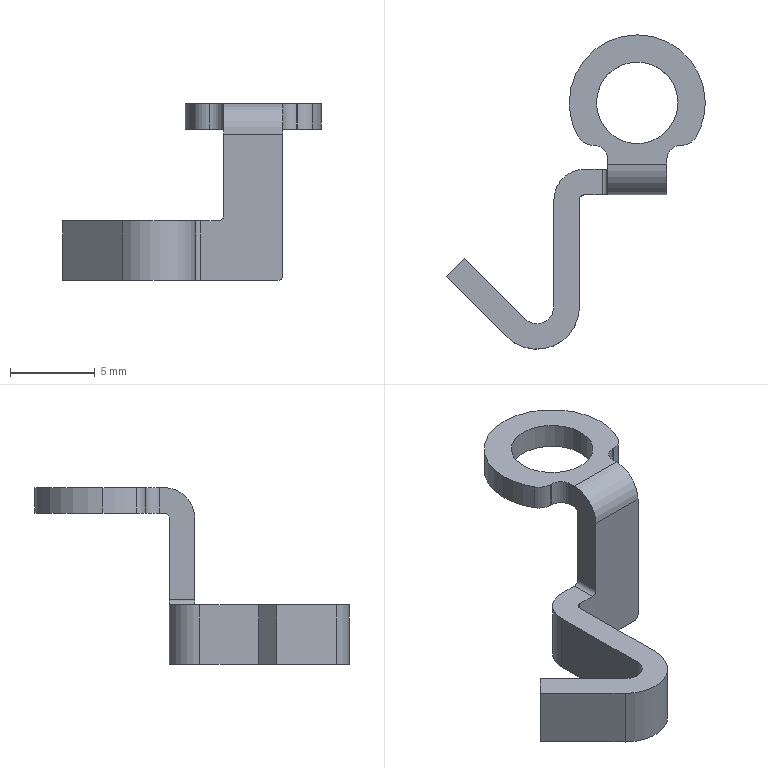Part | STEP file | TQ-DD-1105-THTerminalB1010_デフォルト | 1 solid | 32 faces | box 15.207 x 18.483 x 10.4 mm | volume 194.982 mm3 | cylinder 17 | plane 15 | commonest cylinder face diameters 0.6 x4 2 x3 8 x3 1.6 x2 3.6 x2 4.8 x2
STEP:
#1=CARTESIAN_POINT('',(2.4,0.,0.));
#2=VERTEX_POINT('',#1);
#3=CARTESIAN_POINT('',(-2.4,0.,0.));
#4=VERTEX_POINT('',#3);
#5=CARTESIAN_POINT('',(0.,0.,0.));
#6=DIRECTION('',(0.,0.,-1.));
#7=DIRECTION('',(1.,0.,0.));
#8=AXIS2_PLACEMENT_3D('',#5,#6,#7);
#9=CIRCLE('',#8,2.4);
#10=EDGE_CURVE('',#2,#4,#9,.T.);
#11=ORIENTED_EDGE('',*,*,#10,.T.);
#12=CARTESIAN_POINT('',(-2.4,0.,1.5));
#13=VERTEX_POINT('',#12);
#14=CARTESIAN_POINT('',(-2.4,0.,0.75));
#15=DIRECTION('',(0.,0.,1.));
#16=VECTOR('',#15,1000.);
#17=LINE('',#14,#16);
#18=EDGE_CURVE('',#4,#13,#17,.T.);
#19=ORIENTED_EDGE('',*,*,#18,.T.);
#20=CARTESIAN_POINT('',(2.4,0.,1.5));
#21=VERTEX_POINT('',#20);
#22=CARTESIAN_POINT('',(0.,0.,1.5));
#23=DIRECTION('',(0.,0.,-1.));
#24=DIRECTION('',(1.,0.,0.));
#25=AXIS2_PLACEMENT_3D('',#22,#23,#24);
#26=CIRCLE('',#25,2.4);
#27=EDGE_CURVE('',#21,#13,#26,.T.);
#28=ORIENTED_EDGE('',*,*,#27,.F.);
#29=CARTESIAN_POINT('',(2.4,0.,0.75));
#30=DIRECTION('',(0.,0.,1.));
#31=VECTOR('',#30,1000.);
#32=LINE('',#29,#31);
#33=EDGE_CURVE('',#2,#21,#32,.T.);
#34=ORIENTED_EDGE('',*,*,#33,.F.);
#35=EDGE_LOOP('',(#11,#19,#28,#34));
#36=FACE_OUTER_BOUND('',#35,.T.);
#37=CARTESIAN_POINT('',(0.,0.,0.75));
#38=DIRECTION('',(0.,0.,1.));
#39=DIRECTION('',(1.,0.,0.));
#40=AXIS2_PLACEMENT_3D('',#37,#38,#39);
#41=CYLINDRICAL_SURFACE('',#40,2.4);
#42=ADVANCED_FACE('',(#36),#41,.F.);
#43=CARTESIAN_POINT('',(4.,0.,0.));
#44=VERTEX_POINT('',#43);
#45=CARTESIAN_POINT('',(-4.,0.,0.));
#46=VERTEX_POINT('',#45);
#47=CARTESIAN_POINT('',(0.,0.,0.));
#48=DIRECTION('',(0.,0.,1.));
#49=DIRECTION('',(1.,0.,0.));
#50=AXIS2_PLACEMENT_3D('',#47,#48,#49);
#51=CIRCLE('',#50,4.);
#52=EDGE_CURVE('',#44,#46,#51,.T.);
#53=ORIENTED_EDGE('',*,*,#52,.T.);
#54=CARTESIAN_POINT('',(-4.,0.,1.5));
#55=VERTEX_POINT('',#54);
#56=CARTESIAN_POINT('',(-4.,0.,0.75));
#57=DIRECTION('',(0.,0.,1.));
#58=VECTOR('',#57,1000.);
#59=LINE('',#56,#58);
#60=EDGE_CURVE('',#46,#55,#59,.T.);
#61=ORIENTED_EDGE('',*,*,#60,.T.);
#62=CARTESIAN_POINT('',(4.,0.,1.5));
#63=VERTEX_POINT('',#62);
#64=CARTESIAN_POINT('',(0.,0.,1.5));
#65=DIRECTION('',(0.,0.,1.));
#66=DIRECTION('',(1.,0.,0.));
#67=AXIS2_PLACEMENT_3D('',#64,#65,#66);
#68=CIRCLE('',#67,4.);
#69=EDGE_CURVE('',#63,#55,#68,.T.);
#70=ORIENTED_EDGE('',*,*,#69,.F.);
#71=CARTESIAN_POINT('',(4.,0.,0.75));
#72=DIRECTION('',(0.,0.,1.));
#73=VECTOR('',#72,1000.);
#74=LINE('',#71,#73);
#75=EDGE_CURVE('',#44,#63,#74,.T.);
#76=ORIENTED_EDGE('',*,*,#75,.F.);
#77=EDGE_LOOP('',(#53,#61,#70,#76));
#78=FACE_OUTER_BOUND('',#77,.T.);
#79=CARTESIAN_POINT('',(0.,0.,0.75));
#80=DIRECTION('',(0.,0.,1.));
#81=DIRECTION('',(1.,0.,0.));
#82=AXIS2_PLACEMENT_3D('',#79,#80,#81);
#83=CYLINDRICAL_SURFACE('',#82,4.);
#84=ADVANCED_FACE('',(#78),#83,.T.);
#85=CARTESIAN_POINT('',(3.464,-2.,0.));
#86=VERTEX_POINT('',#85);
#87=CARTESIAN_POINT('',(0.,0.,0.));
#88=DIRECTION('',(0.,0.,1.));
#89=DIRECTION('',(1.,0.,0.));
#90=AXIS2_PLACEMENT_3D('',#87,#88,#89);
#91=CIRCLE('',#90,4.);
#92=EDGE_CURVE('',#86,#44,#91,.T.);
#93=ORIENTED_EDGE('',*,*,#92,.T.);
#94=ORIENTED_EDGE('',*,*,#75,.T.);
#95=CARTESIAN_POINT('',(3.464,-2.,1.5));
#96=VERTEX_POINT('',#95);
#97=CARTESIAN_POINT('',(0.,0.,1.5));
#98=DIRECTION('',(0.,0.,1.));
#99=DIRECTION('',(1.,0.,0.));
#100=AXIS2_PLACEMENT_3D('',#97,#98,#99);
#101=CIRCLE('',#100,4.);
#102=EDGE_CURVE('',#96,#63,#101,.T.);
#103=ORIENTED_EDGE('',*,*,#102,.F.);
#104=CARTESIAN_POINT('',(3.464,-2.,0.75));
#105=DIRECTION('',(0.,0.,1.));
#106=VECTOR('',#105,1000.);
#107=LINE('',#104,#106);
#108=EDGE_CURVE('',#86,#96,#107,.T.);
#109=ORIENTED_EDGE('',*,*,#108,.F.);
#110=EDGE_LOOP('',(#93,#94,#103,#109));
#111=FACE_OUTER_BOUND('',#110,.T.);
#112=CARTESIAN_POINT('',(0.,0.,0.75));
#113=DIRECTION('',(0.,0.,1.));
#114=DIRECTION('',(1.,0.,0.));
#115=AXIS2_PLACEMENT_3D('',#112,#113,#114);
#116=CYLINDRICAL_SURFACE('',#115,4.);
#117=ADVANCED_FACE('',(#111),#116,.T.);
#118=CARTESIAN_POINT('',(-3.104,-3.9,-8.9));
#119=VERTEX_POINT('',#118);
#120=CARTESIAN_POINT('',(1.45,-3.9,-8.9));
#121=VERTEX_POINT('',#120);
#122=CARTESIAN_POINT('',(0.,-3.9,-8.9));
#123=DIRECTION('',(1.,0.,0.));
#124=VECTOR('',#123,1000.);
#125=LINE('',#122,#124);
#126=EDGE_CURVE('',#119,#121,#125,.T.);
#127=ORIENTED_EDGE('',*,*,#126,.F.);
#128=CARTESIAN_POINT('',(-3.104,-3.9,-5.4));
#129=VERTEX_POINT('',#128);
#130=CARTESIAN_POINT('',(-3.104,-3.9,1.5));
#131=DIRECTION('',(0.,0.,-1.));
#132=VECTOR('',#131,1000.);
#133=LINE('',#130,#132);
#134=EDGE_CURVE('',#129,#119,#133,.T.);
#135=ORIENTED_EDGE('',*,*,#134,.F.);
#136=CARTESIAN_POINT('',(-2.05,-3.9,-5.4));
#137=VERTEX_POINT('',#136);
#138=CARTESIAN_POINT('',(0.,-3.9,-5.4));
#139=DIRECTION('',(1.,0.,0.));
#140=VECTOR('',#139,1000.);
#141=LINE('',#138,#140);
#142=EDGE_CURVE('',#129,#137,#141,.T.);
#143=ORIENTED_EDGE('',*,*,#142,.T.);
#144=CARTESIAN_POINT('',(-1.75,-3.9,-5.1));
#145=VERTEX_POINT('',#144);
#146=CARTESIAN_POINT('',(-2.05,-3.9,-5.1));
#147=DIRECTION('',(0.,-1.,0.));
#148=DIRECTION('',(0.,0.,1.));
#149=AXIS2_PLACEMENT_3D('',#146,#147,#148);
#150=CIRCLE('',#149,0.3);
#151=EDGE_CURVE('',#137,#145,#150,.T.);
#152=ORIENTED_EDGE('',*,*,#151,.T.);
#153=CARTESIAN_POINT('',(-1.75,-3.9,-0.3));
#154=VERTEX_POINT('',#153);
#155=CARTESIAN_POINT('',(-1.75,-3.9,1.5));
#156=DIRECTION('',(0.,0.,-1.));
#157=VECTOR('',#156,1000.);
#158=LINE('',#155,#157);
#159=EDGE_CURVE('',#154,#145,#158,.T.);
#160=ORIENTED_EDGE('',*,*,#159,.F.);
#161=CARTESIAN_POINT('',(1.75,-3.9,-0.3));
#162=VERTEX_POINT('',#161);
#163=CARTESIAN_POINT('',(0.,-3.9,-0.3));
#164=DIRECTION('',(-1.,0.,0.));
#165=VECTOR('',#164,1000.);
#166=LINE('',#163,#165);
#167=EDGE_CURVE('',#162,#154,#166,.T.);
#168=ORIENTED_EDGE('',*,*,#167,.F.);
#169=CARTESIAN_POINT('',(1.75,-3.9,-8.6));
#170=VERTEX_POINT('',#169);
#171=CARTESIAN_POINT('',(1.75,-3.9,1.5));
#172=DIRECTION('',(0.,0.,1.));
#173=VECTOR('',#172,1000.);
#174=LINE('',#171,#173);
#175=EDGE_CURVE('',#170,#162,#174,.T.);
#176=ORIENTED_EDGE('',*,*,#175,.F.);
#177=CARTESIAN_POINT('',(1.45,-3.9,-8.6));
#178=DIRECTION('',(0.,-1.,0.));
#179=DIRECTION('',(0.,0.,1.));
#180=AXIS2_PLACEMENT_3D('',#177,#178,#179);
#181=CIRCLE('',#180,0.3);
#182=EDGE_CURVE('',#121,#170,#181,.T.);
#183=ORIENTED_EDGE('',*,*,#182,.F.);
#184=EDGE_LOOP('',(#127,#135,#143,#152,#160,#168,#176,#183));
#185=FACE_OUTER_BOUND('',#184,.T.);
#186=CARTESIAN_POINT('',(0.,-3.9,1.5));
#187=DIRECTION('',(0.,-1.,0.));
#188=DIRECTION('',(0.,0.,-1.));
#189=AXIS2_PLACEMENT_3D('',#186,#187,#188);
#190=PLANE('',#189);
#191=ADVANCED_FACE('',(#185),#190,.F.);
#192=ORIENTED_EDGE('',*,*,#126,.T.);
#193=CARTESIAN_POINT('',(1.45,-5.4,-8.9));
#194=VERTEX_POINT('',#193);
#195=CARTESIAN_POINT('',(1.45,-5.4,-8.9));
#196=DIRECTION('',(0.,-1.,0.));
#197=VECTOR('',#196,1000.);
#198=LINE('',#195,#197);
#199=EDGE_CURVE('',#121,#194,#198,.T.);
#200=ORIENTED_EDGE('',*,*,#199,.T.);
#201=CARTESIAN_POINT('',(-3.104,-5.4,-8.9));
#202=VERTEX_POINT('',#201);
#203=CARTESIAN_POINT('',(0.,-5.4,-8.9));
#204=DIRECTION('',(-1.,0.,0.));
#205=VECTOR('',#204,1000.);
#206=LINE('',#203,#205);
#207=EDGE_CURVE('',#194,#202,#206,.T.);
#208=ORIENTED_EDGE('',*,*,#207,.T.);
#209=CARTESIAN_POINT('',(-3.404,-5.7,-8.9));
#210=VERTEX_POINT('',#209);
#211=CARTESIAN_POINT('',(-3.104,-5.7,-8.9));
#212=DIRECTION('',(0.,0.,1.));
#213=DIRECTION('',(-1.,0.,0.));
#214=AXIS2_PLACEMENT_3D('',#211,#212,#213);
#215=CIRCLE('',#214,0.3);
#216=EDGE_CURVE('',#202,#210,#215,.T.);
#217=ORIENTED_EDGE('',*,*,#216,.T.);
#218=CARTESIAN_POINT('',(-3.404,-11.983,-8.9));
#219=VERTEX_POINT('',#218);
#220=CARTESIAN_POINT('',(-3.404,-5.4,-8.9));
#221=DIRECTION('',(0.,-1.,0.));
#222=VECTOR('',#221,1000.);
#223=LINE('',#220,#222);
#224=EDGE_CURVE('',#210,#219,#223,.T.);
#225=ORIENTED_EDGE('',*,*,#224,.T.);
#226=CARTESIAN_POINT('',(-7.672,-13.751,-8.9));
#227=VERTEX_POINT('',#226);
#228=CARTESIAN_POINT('',(-5.904,-11.983,-8.9));
#229=DIRECTION('',(0.,0.,-1.));
#230=DIRECTION('',(-1.,0.,0.));
#231=AXIS2_PLACEMENT_3D('',#228,#229,#230);
#232=CIRCLE('',#231,2.5);
#233=EDGE_CURVE('',#219,#227,#232,.T.);
#234=ORIENTED_EDGE('',*,*,#233,.T.);
#235=CARTESIAN_POINT('',(-11.207,-10.216,-8.9));
#236=VERTEX_POINT('',#235);
#237=CARTESIAN_POINT('',(-7.672,-13.751,-8.9));
#238=DIRECTION('',(-0.7071,0.7071,0.));
#239=VECTOR('',#238,1000.);
#240=LINE('',#237,#239);
#241=EDGE_CURVE('',#227,#236,#240,.T.);
#242=ORIENTED_EDGE('',*,*,#241,.T.);
#243=CARTESIAN_POINT('',(-10.147,-9.155,-8.9));
#244=VERTEX_POINT('',#243);
#245=CARTESIAN_POINT('',(-10.147,-9.155,-8.9));
#246=DIRECTION('',(-0.7071,-0.7071,0.));
#247=VECTOR('',#246,1000.);
#248=LINE('',#245,#247);
#249=EDGE_CURVE('',#244,#236,#248,.T.);
#250=ORIENTED_EDGE('',*,*,#249,.F.);
#251=CARTESIAN_POINT('',(-6.611,-12.691,-8.9));
#252=VERTEX_POINT('',#251);
#253=CARTESIAN_POINT('',(-10.147,-9.155,-8.9));
#254=DIRECTION('',(0.7071,-0.7071,0.));
#255=VECTOR('',#254,1000.);
#256=LINE('',#253,#255);
#257=EDGE_CURVE('',#244,#252,#256,.T.);
#258=ORIENTED_EDGE('',*,*,#257,.T.);
#259=CARTESIAN_POINT('',(-4.904,-11.983,-8.9));
#260=VERTEX_POINT('',#259);
#261=CARTESIAN_POINT('',(-5.904,-11.983,-8.9));
#262=DIRECTION('',(0.,0.,1.));
#263=DIRECTION('',(-1.,0.,0.));
#264=AXIS2_PLACEMENT_3D('',#261,#262,#263);
#265=CIRCLE('',#264,1.);
#266=EDGE_CURVE('',#252,#260,#265,.T.);
#267=ORIENTED_EDGE('',*,*,#266,.T.);
#268=CARTESIAN_POINT('',(-4.904,-5.7,-8.9));
#269=VERTEX_POINT('',#268);
#270=CARTESIAN_POINT('',(-4.904,-5.4,-8.9));
#271=DIRECTION('',(0.,1.,0.));
#272=VECTOR('',#271,1000.);
#273=LINE('',#270,#272);
#274=EDGE_CURVE('',#260,#269,#273,.T.);
#275=ORIENTED_EDGE('',*,*,#274,.T.);
#276=CARTESIAN_POINT('',(-3.104,-5.7,-8.9));
#277=DIRECTION('',(0.,0.,-1.));
#278=DIRECTION('',(-1.,0.,0.));
#279=AXIS2_PLACEMENT_3D('',#276,#277,#278);
#280=CIRCLE('',#279,1.8);
#281=EDGE_CURVE('',#269,#119,#280,.T.);
#282=ORIENTED_EDGE('',*,*,#281,.T.);
#283=EDGE_LOOP('',(#192,#200,#208,#217,#225,#234,#242,#250,#258,#267,#275,#282));
#284=FACE_OUTER_BOUND('',#283,.T.);
#285=CARTESIAN_POINT('',(0.,-5.4,-8.9));
#286=DIRECTION('',(0.,0.,-1.));
#287=DIRECTION('',(-1.,0.,0.));
#288=AXIS2_PLACEMENT_3D('',#285,#286,#287);
#289=PLANE('',#288);
#290=ADVANCED_FACE('',(#284),#289,.T.);
#291=ORIENTED_EDGE('',*,*,#281,.F.);
#292=CARTESIAN_POINT('',(-4.904,-5.7,-5.4));
#293=VERTEX_POINT('',#292);
#294=CARTESIAN_POINT('',(-4.904,-5.7,-7.15));
#295=DIRECTION('',(0.,0.,1.));
#296=VECTOR('',#295,1000.);
#297=LINE('',#294,#296);
#298=EDGE_CURVE('',#269,#293,#297,.T.);
#299=ORIENTED_EDGE('',*,*,#298,.T.);
#300=CARTESIAN_POINT('',(-3.104,-5.7,-5.4));
#301=DIRECTION('',(0.,0.,-1.));
#302=DIRECTION('',(-1.,0.,0.));
#303=AXIS2_PLACEMENT_3D('',#300,#301,#302);
#304=CIRCLE('',#303,1.8);
#305=EDGE_CURVE('',#293,#129,#304,.T.);
#306=ORIENTED_EDGE('',*,*,#305,.T.);
#307=ORIENTED_EDGE('',*,*,#134,.T.);
#308=EDGE_LOOP('',(#291,#299,#306,#307));
#309=FACE_OUTER_BOUND('',#308,.T.);
#310=CARTESIAN_POINT('',(-3.104,-5.7,-7.15));
#311=DIRECTION('',(0.,0.,-1.));
#312=DIRECTION('',(-1.,0.,0.));
#313=AXIS2_PLACEMENT_3D('',#310,#311,#312);
#314=CYLINDRICAL_SURFACE('',#313,1.8);
#315=ADVANCED_FACE('',(#309),#314,.T.);
#316=ORIENTED_EDGE('',*,*,#159,.T.);
#317=CARTESIAN_POINT('',(-1.75,-5.4,-5.1));
#318=VERTEX_POINT('',#317);
#319=CARTESIAN_POINT('',(-1.75,-2.5,-5.1));
#320=DIRECTION('',(0.,-1.,0.));
#321=VECTOR('',#320,1000.);
#322=LINE('',#319,#321);
#323=EDGE_CURVE('',#145,#318,#322,.T.);
#324=ORIENTED_EDGE('',*,*,#323,.T.);
#325=CARTESIAN_POINT('',(-1.75,-5.4,-0.3));
#326=VERTEX_POINT('',#325);
#327=CARTESIAN_POINT('',(-1.75,-5.4,0.));
#328=DIRECTION('',(0.,0.,1.));
#329=VECTOR('',#328,1000.);
#330=LINE('',#327,#329);
#331=EDGE_CURVE('',#318,#326,#330,.T.);
#332=ORIENTED_EDGE('',*,*,#331,.T.);
#333=CARTESIAN_POINT('',(-1.75,-3.6,1.5));
#334=VERTEX_POINT('',#333);
#335=CARTESIAN_POINT('',(-1.75,-3.6,-0.3));
#336=DIRECTION('',(-1.,0.,0.));
#337=DIRECTION('',(0.,0.,-1.));
#338=AXIS2_PLACEMENT_3D('',#335,#336,#337);
#339=CIRCLE('',#338,1.8);
#340=EDGE_CURVE('',#326,#334,#339,.T.);
#341=ORIENTED_EDGE('',*,*,#340,.T.);
#342=CARTESIAN_POINT('',(-1.75,-3.3,1.5));
#343=VERTEX_POINT('',#342);
#344=CARTESIAN_POINT('',(-1.75,0.,1.5));
#345=DIRECTION('',(0.,-1.,0.));
#346=VECTOR('',#345,1000.);
#347=LINE('',#344,#346);
#348=EDGE_CURVE('',#343,#334,#347,.T.);
#349=ORIENTED_EDGE('',*,*,#348,.F.);
#350=CARTESIAN_POINT('',(-1.75,-3.3,0.));
#351=VERTEX_POINT('',#350);
#352=CARTESIAN_POINT('',(-1.75,-3.3,0.));
#353=DIRECTION('',(0.,0.,-1.));
#354=VECTOR('',#353,1000.);
#355=LINE('',#352,#354);
#356=EDGE_CURVE('',#343,#351,#355,.T.);
#357=ORIENTED_EDGE('',*,*,#356,.T.);
#358=CARTESIAN_POINT('',(-1.75,-3.6,0.));
#359=VERTEX_POINT('',#358);
#360=CARTESIAN_POINT('',(-1.75,0.,0.));
#361=DIRECTION('',(0.,-1.,0.));
#362=VECTOR('',#361,1000.);
#363=LINE('',#360,#362);
#364=EDGE_CURVE('',#351,#359,#363,.T.);
#365=ORIENTED_EDGE('',*,*,#364,.T.);
#366=CARTESIAN_POINT('',(-1.75,-3.6,-0.3));
#367=DIRECTION('',(1.,0.,0.));
#368=DIRECTION('',(0.,0.,1.));
#369=AXIS2_PLACEMENT_3D('',#366,#367,#368);
#370=CIRCLE('',#369,0.3);
#371=EDGE_CURVE('',#359,#154,#370,.T.);
#372=ORIENTED_EDGE('',*,*,#371,.T.);
#373=EDGE_LOOP('',(#316,#324,#332,#341,#349,#357,#365,#372));
#374=FACE_OUTER_BOUND('',#373,.T.);
#375=CARTESIAN_POINT('',(-1.75,-2.5,0.));
#376=DIRECTION('',(-1.,0.,0.));
#377=DIRECTION('',(0.,0.,1.));
#378=AXIS2_PLACEMENT_3D('',#375,#376,#377);
#379=PLANE('',#378);
#380=ADVANCED_FACE('',(#374),#379,.T.);
#381=ORIENTED_EDGE('',*,*,#371,.F.);
#382=CARTESIAN_POINT('',(1.75,-3.6,0.));
#383=VERTEX_POINT('',#382);
#384=CARTESIAN_POINT('',(0.,-3.6,0.));
#385=DIRECTION('',(-1.,0.,0.));
#386=VECTOR('',#385,1000.);
#387=LINE('',#384,#386);
#388=EDGE_CURVE('',#383,#359,#387,.T.);
#389=ORIENTED_EDGE('',*,*,#388,.F.);
#390=CARTESIAN_POINT('',(1.75,-3.6,-0.3));
#391=DIRECTION('',(-1.,0.,0.));
#392=DIRECTION('',(0.,0.,1.));
#393=AXIS2_PLACEMENT_3D('',#390,#391,#392);
#394=CIRCLE('',#393,0.3);
#395=EDGE_CURVE('',#162,#383,#394,.T.);
#396=ORIENTED_EDGE('',*,*,#395,.F.);
#397=ORIENTED_EDGE('',*,*,#167,.T.);
#398=EDGE_LOOP('',(#381,#389,#396,#397));
#399=FACE_OUTER_BOUND('',#398,.T.);
#400=CARTESIAN_POINT('',(0.,-3.6,-0.3));
#401=DIRECTION('',(-1.,0.,0.));
#402=DIRECTION('',(0.,0.,1.));
#403=AXIS2_PLACEMENT_3D('',#400,#401,#402);
#404=CYLINDRICAL_SURFACE('',#403,0.3);
#405=ADVANCED_FACE('',(#399),#404,.F.);
#406=CARTESIAN_POINT('',(1.75,-5.4,-0.3));
#407=VERTEX_POINT('',#406);
#408=CARTESIAN_POINT('',(1.75,-5.4,-8.6));
#409=VERTEX_POINT('',#408);
#410=CARTESIAN_POINT('',(1.75,-5.4,0.));
#411=DIRECTION('',(0.,0.,-1.));
#412=VECTOR('',#411,1000.);
#413=LINE('',#410,#412);
#414=EDGE_CURVE('',#407,#409,#413,.T.);
#415=ORIENTED_EDGE('',*,*,#414,.T.);
#416=CARTESIAN_POINT('',(1.75,-5.4,-8.6));
#417=DIRECTION('',(0.,1.,0.));
#418=VECTOR('',#417,1000.);
#419=LINE('',#416,#418);
#420=EDGE_CURVE('',#409,#170,#419,.T.);
#421=ORIENTED_EDGE('',*,*,#420,.T.);
#422=ORIENTED_EDGE('',*,*,#175,.T.);
#423=ORIENTED_EDGE('',*,*,#395,.T.);
#424=CARTESIAN_POINT('',(1.75,-3.3,0.));
#425=VERTEX_POINT('',#424);
#426=CARTESIAN_POINT('',(1.75,-5.4,0.));
#427=DIRECTION('',(0.,1.,0.));
#428=VECTOR('',#427,1000.);
#429=LINE('',#426,#428);
#430=EDGE_CURVE('',#383,#425,#429,.T.);
#431=ORIENTED_EDGE('',*,*,#430,.T.);
#432=CARTESIAN_POINT('',(1.75,-3.3,1.5));
#433=VERTEX_POINT('',#432);
#434=CARTESIAN_POINT('',(1.75,-3.3,0.));
#435=DIRECTION('',(0.,0.,1.));
#436=VECTOR('',#435,1000.);
#437=LINE('',#434,#436);
#438=EDGE_CURVE('',#425,#433,#437,.T.);
#439=ORIENTED_EDGE('',*,*,#438,.T.);
#440=CARTESIAN_POINT('',(1.75,-3.6,1.5));
#441=VERTEX_POINT('',#440);
#442=CARTESIAN_POINT('',(1.75,0.,1.5));
#443=DIRECTION('',(0.,1.,0.));
#444=VECTOR('',#443,1000.);
#445=LINE('',#442,#444);
#446=EDGE_CURVE('',#441,#433,#445,.T.);
#447=ORIENTED_EDGE('',*,*,#446,.F.);
#448=CARTESIAN_POINT('',(1.75,-3.6,-0.3));
#449=DIRECTION('',(1.,0.,0.));
#450=DIRECTION('',(0.,0.,-1.));
#451=AXIS2_PLACEMENT_3D('',#448,#449,#450);
#452=CIRCLE('',#451,1.8);
#453=EDGE_CURVE('',#441,#407,#452,.T.);
#454=ORIENTED_EDGE('',*,*,#453,.T.);
#455=EDGE_LOOP('',(#415,#421,#422,#423,#431,#439,#447,#454));
#456=FACE_OUTER_BOUND('',#455,.T.);
#457=CARTESIAN_POINT('',(1.75,-5.4,0.));
#458=DIRECTION('',(1.,0.,0.));
#459=DIRECTION('',(0.,0.,-1.));
#460=AXIS2_PLACEMENT_3D('',#457,#458,#459);
#461=PLANE('',#460);
#462=ADVANCED_FACE('',(#456),#461,.T.);
#463=CARTESIAN_POINT('',(1.45,-5.4,-8.6));
#464=DIRECTION('',(0.,1.,0.));
#465=DIRECTION('',(0.,0.,1.));
#466=AXIS2_PLACEMENT_3D('',#463,#464,#465);
#467=CIRCLE('',#466,0.3);
#468=EDGE_CURVE('',#409,#194,#467,.T.);
#469=ORIENTED_EDGE('',*,*,#468,.T.);
#470=ORIENTED_EDGE('',*,*,#199,.F.);
#471=ORIENTED_EDGE('',*,*,#182,.T.);
#472=ORIENTED_EDGE('',*,*,#420,.F.);
#473=EDGE_LOOP('',(#469,#470,#471,#472));
#474=FACE_OUTER_BOUND('',#473,.T.);
#475=CARTESIAN_POINT('',(1.45,-9.192,-8.6));
#476=DIRECTION('',(0.,1.,0.));
#477=DIRECTION('',(0.,0.,1.));
#478=AXIS2_PLACEMENT_3D('',#475,#476,#477);
#479=CYLINDRICAL_SURFACE('',#478,0.3);
#480=ADVANCED_FACE('',(#474),#479,.T.);
#481=ORIENTED_EDGE('',*,*,#274,.F.);
#482=CARTESIAN_POINT('',(-4.904,-11.983,-5.4));
#483=VERTEX_POINT('',#482);
#484=CARTESIAN_POINT('',(-4.904,-11.983,-8.9));
#485=DIRECTION('',(0.,0.,1.));
#486=VECTOR('',#485,1000.);
#487=LINE('',#484,#486);
#488=EDGE_CURVE('',#260,#483,#487,.T.);
#489=ORIENTED_EDGE('',*,*,#488,.T.);
#490=CARTESIAN_POINT('',(-4.904,-5.7,-5.4));
#491=DIRECTION('',(0.,1.,0.));
#492=VECTOR('',#491,1000.);
#493=LINE('',#490,#492);
#494=EDGE_CURVE('',#483,#293,#493,.T.);
#495=ORIENTED_EDGE('',*,*,#494,.T.);
#496=ORIENTED_EDGE('',*,*,#298,.F.);
#497=EDGE_LOOP('',(#481,#489,#495,#496));
#498=FACE_OUTER_BOUND('',#497,.T.);
#499=CARTESIAN_POINT('',(-4.904,-5.7,-8.9));
#500=DIRECTION('',(-1.,0.,0.));
#501=DIRECTION('',(0.,0.,1.));
#502=AXIS2_PLACEMENT_3D('',#499,#500,#501);
#503=PLANE('',#502);
#504=ADVANCED_FACE('',(#498),#503,.T.);
#505=ORIENTED_EDGE('',*,*,#488,.F.);
#506=ORIENTED_EDGE('',*,*,#266,.F.);
#507=CARTESIAN_POINT('',(-6.611,-12.691,-5.4));
#508=VERTEX_POINT('',#507);
#509=CARTESIAN_POINT('',(-6.611,-12.691,-7.15));
#510=DIRECTION('',(0.,0.,-1.));
#511=VECTOR('',#510,1000.);
#512=LINE('',#509,#511);
#513=EDGE_CURVE('',#508,#252,#512,.T.);
#514=ORIENTED_EDGE('',*,*,#513,.F.);
#515=CARTESIAN_POINT('',(-5.904,-11.983,-5.4));
#516=DIRECTION('',(0.,0.,-1.));
#517=DIRECTION('',(-1.,0.,0.));
#518=AXIS2_PLACEMENT_3D('',#515,#516,#517);
#519=CIRCLE('',#518,1.);
#520=EDGE_CURVE('',#483,#508,#519,.T.);
#521=ORIENTED_EDGE('',*,*,#520,.F.);
#522=EDGE_LOOP('',(#505,#506,#514,#521));
#523=FACE_OUTER_BOUND('',#522,.T.);
#524=CARTESIAN_POINT('',(-5.904,-11.983,-7.15));
#525=DIRECTION('',(0.,0.,-1.));
#526=DIRECTION('',(-1.,0.,0.));
#527=AXIS2_PLACEMENT_3D('',#524,#525,#526);
#528=CYLINDRICAL_SURFACE('',#527,1.);
#529=ADVANCED_FACE('',(#523),#528,.F.);
#530=ORIENTED_EDGE('',*,*,#513,.T.);
#531=ORIENTED_EDGE('',*,*,#257,.F.);
#532=CARTESIAN_POINT('',(-10.147,-9.155,-5.4));
#533=VERTEX_POINT('',#532);
#534=CARTESIAN_POINT('',(-10.147,-9.155,-8.9));
#535=DIRECTION('',(0.,0.,-1.));
#536=VECTOR('',#535,1000.);
#537=LINE('',#534,#536);
#538=EDGE_CURVE('',#533,#244,#537,.T.);
#539=ORIENTED_EDGE('',*,*,#538,.F.);
#540=CARTESIAN_POINT('',(-10.147,-9.155,-5.4));
#541=DIRECTION('',(-0.7071,0.7071,0.));
#542=VECTOR('',#541,1000.);
#543=LINE('',#540,#542);
#544=EDGE_CURVE('',#508,#533,#543,.T.);
#545=ORIENTED_EDGE('',*,*,#544,.F.);
#546=EDGE_LOOP('',(#530,#531,#539,#545));
#547=FACE_OUTER_BOUND('',#546,.T.);
#548=CARTESIAN_POINT('',(-10.147,-9.155,-8.9));
#549=DIRECTION('',(-0.7071,-0.7071,0.));
#550=DIRECTION('',(0.7071,-0.7071,0.));
#551=AXIS2_PLACEMENT_3D('',#548,#549,#550);
#552=PLANE('',#551);
#553=ADVANCED_FACE('',(#547),#552,.F.);
#554=ORIENTED_EDGE('',*,*,#241,.F.);
#555=CARTESIAN_POINT('',(-7.672,-13.751,-5.4));
#556=VERTEX_POINT('',#555);
#557=CARTESIAN_POINT('',(-7.672,-13.751,-8.9));
#558=DIRECTION('',(0.,0.,1.));
#559=VECTOR('',#558,1000.);
#560=LINE('',#557,#559);
#561=EDGE_CURVE('',#227,#556,#560,.T.);
#562=ORIENTED_EDGE('',*,*,#561,.T.);
#563=CARTESIAN_POINT('',(-11.207,-10.216,-5.4));
#564=VERTEX_POINT('',#563);
#565=CARTESIAN_POINT('',(-11.207,-10.216,-5.4));
#566=DIRECTION('',(-0.7071,0.7071,0.));
#567=VECTOR('',#566,1000.);
#568=LINE('',#565,#567);
#569=EDGE_CURVE('',#556,#564,#568,.T.);
#570=ORIENTED_EDGE('',*,*,#569,.T.);
#571=CARTESIAN_POINT('',(-11.207,-10.216,-8.9));
#572=DIRECTION('',(0.,0.,-1.));
#573=VECTOR('',#572,1000.);
#574=LINE('',#571,#573);
#575=EDGE_CURVE('',#564,#236,#574,.T.);
#576=ORIENTED_EDGE('',*,*,#575,.T.);
#577=EDGE_LOOP('',(#554,#562,#570,#576));
#578=FACE_OUTER_BOUND('',#577,.T.);
#579=CARTESIAN_POINT('',(-11.207,-10.216,-8.9));
#580=DIRECTION('',(-0.7071,-0.7071,0.));
#581=DIRECTION('',(0.7071,-0.7071,0.));
#582=AXIS2_PLACEMENT_3D('',#579,#580,#581);
#583=PLANE('',#582);
#584=ADVANCED_FACE('',(#578),#583,.T.);
#585=ORIENTED_EDGE('',*,*,#233,.F.);
#586=CARTESIAN_POINT('',(-3.404,-11.983,-5.4));
#587=VERTEX_POINT('',#586);
#588=CARTESIAN_POINT('',(-3.404,-11.983,-7.15));
#589=DIRECTION('',(0.,0.,1.));
#590=VECTOR('',#589,1000.);
#591=LINE('',#588,#590);
#592=EDGE_CURVE('',#219,#587,#591,.T.);
#593=ORIENTED_EDGE('',*,*,#592,.T.);
#594=CARTESIAN_POINT('',(-5.904,-11.983,-5.4));
#595=DIRECTION('',(0.,0.,-1.));
#596=DIRECTION('',(-1.,0.,0.));
#597=AXIS2_PLACEMENT_3D('',#594,#595,#596);
#598=CIRCLE('',#597,2.5);
#599=EDGE_CURVE('',#587,#556,#598,.T.);
#600=ORIENTED_EDGE('',*,*,#599,.T.);
#601=ORIENTED_EDGE('',*,*,#561,.F.);
#602=EDGE_LOOP('',(#585,#593,#600,#601));
#603=FACE_OUTER_BOUND('',#602,.T.);
#604=CARTESIAN_POINT('',(-5.904,-11.983,-7.15));
#605=DIRECTION('',(0.,0.,-1.));
#606=DIRECTION('',(-1.,0.,0.));
#607=AXIS2_PLACEMENT_3D('',#604,#605,#606);
#608=CYLINDRICAL_SURFACE('',#607,2.5);
#609=ADVANCED_FACE('',(#603),#608,.T.);
#610=ORIENTED_EDGE('',*,*,#592,.F.);
#611=ORIENTED_EDGE('',*,*,#224,.F.);
#612=CARTESIAN_POINT('',(-3.404,-5.7,-5.4));
#613=VERTEX_POINT('',#612);
#614=CARTESIAN_POINT('',(-3.404,-5.7,-8.9));
#615=DIRECTION('',(0.,0.,-1.));
#616=VECTOR('',#615,1000.);
#617=LINE('',#614,#616);
#618=EDGE_CURVE('',#613,#210,#617,.T.);
#619=ORIENTED_EDGE('',*,*,#618,.F.);
#620=CARTESIAN_POINT('',(-3.404,-5.7,-5.4));
#621=DIRECTION('',(0.,1.,0.));
#622=VECTOR('',#621,1000.);
#623=LINE('',#620,#622);
#624=EDGE_CURVE('',#587,#613,#623,.T.);
#625=ORIENTED_EDGE('',*,*,#624,.F.);
#626=EDGE_LOOP('',(#610,#611,#619,#625));
#627=FACE_OUTER_BOUND('',#626,.T.);
#628=CARTESIAN_POINT('',(-3.404,-5.7,-8.9));
#629=DIRECTION('',(-1.,0.,0.));
#630=DIRECTION('',(0.,0.,1.));
#631=AXIS2_PLACEMENT_3D('',#628,#629,#630);
#632=PLANE('',#631);
#633=ADVANCED_FACE('',(#627),#632,.F.);
#634=ORIENTED_EDGE('',*,*,#207,.F.);
#635=ORIENTED_EDGE('',*,*,#468,.F.);
#636=ORIENTED_EDGE('',*,*,#414,.F.);
#637=CARTESIAN_POINT('',(-1.75,-5.4,-0.3));
#638=DIRECTION('',(-1.,0.,0.));
#639=VECTOR('',#638,1000.);
#640=LINE('',#637,#639);
#641=EDGE_CURVE('',#407,#326,#640,.T.);
#642=ORIENTED_EDGE('',*,*,#641,.T.);
#643=ORIENTED_EDGE('',*,*,#331,.F.);
#644=CARTESIAN_POINT('',(-2.05,-5.4,-5.4));
#645=VERTEX_POINT('',#644);
#646=CARTESIAN_POINT('',(-2.05,-5.4,-5.1));
#647=DIRECTION('',(0.,1.,0.));
#648=DIRECTION('',(0.,0.,1.));
#649=AXIS2_PLACEMENT_3D('',#646,#647,#648);
#650=CIRCLE('',#649,0.3);
#651=EDGE_CURVE('',#318,#645,#650,.T.);
#652=ORIENTED_EDGE('',*,*,#651,.T.);
#653=CARTESIAN_POINT('',(-3.104,-5.4,-5.4));
#654=VERTEX_POINT('',#653);
#655=CARTESIAN_POINT('',(-1.75,-5.4,-5.4));
#656=DIRECTION('',(-1.,0.,0.));
#657=VECTOR('',#656,1000.);
#658=LINE('',#655,#657);
#659=EDGE_CURVE('',#645,#654,#658,.T.);
#660=ORIENTED_EDGE('',*,*,#659,.T.);
#661=CARTESIAN_POINT('',(-3.104,-5.4,0.));
#662=DIRECTION('',(0.,0.,-1.));
#663=VECTOR('',#662,1000.);
#664=LINE('',#661,#663);
#665=EDGE_CURVE('',#654,#202,#664,.T.);
#666=ORIENTED_EDGE('',*,*,#665,.T.);
#667=EDGE_LOOP('',(#634,#635,#636,#642,#643,#652,#660,#666));
#668=FACE_OUTER_BOUND('',#667,.T.);
#669=CARTESIAN_POINT('',(-1.75,-5.4,0.));
#670=DIRECTION('',(0.,-1.,0.));
#671=DIRECTION('',(0.,0.,-1.));
#672=AXIS2_PLACEMENT_3D('',#669,#670,#671);
#673=PLANE('',#672);
#674=ADVANCED_FACE('',(#668),#673,.T.);
#675=ORIENTED_EDGE('',*,*,#142,.F.);
#676=ORIENTED_EDGE('',*,*,#305,.F.);
#677=ORIENTED_EDGE('',*,*,#494,.F.);
#678=ORIENTED_EDGE('',*,*,#520,.T.);
#679=ORIENTED_EDGE('',*,*,#544,.T.);
#680=CARTESIAN_POINT('',(-11.207,-10.216,-5.4));
#681=DIRECTION('',(0.7071,0.7071,0.));
#682=VECTOR('',#681,1000.);
#683=LINE('',#680,#682);
#684=EDGE_CURVE('',#564,#533,#683,.T.);
#685=ORIENTED_EDGE('',*,*,#684,.F.);
#686=ORIENTED_EDGE('',*,*,#569,.F.);
#687=ORIENTED_EDGE('',*,*,#599,.F.);
#688=ORIENTED_EDGE('',*,*,#624,.T.);
#689=CARTESIAN_POINT('',(-3.104,-5.7,-5.4));
#690=DIRECTION('',(0.,0.,1.));
#691=DIRECTION('',(-1.,0.,0.));
#692=AXIS2_PLACEMENT_3D('',#689,#690,#691);
#693=CIRCLE('',#692,0.3);
#694=EDGE_CURVE('',#654,#613,#693,.T.);
#695=ORIENTED_EDGE('',*,*,#694,.F.);
#696=ORIENTED_EDGE('',*,*,#659,.F.);
#697=CARTESIAN_POINT('',(-2.05,0.,-5.4));
#698=DIRECTION('',(0.,-1.,0.));
#699=VECTOR('',#698,1000.);
#700=LINE('',#697,#699);
#701=EDGE_CURVE('',#137,#645,#700,.T.);
#702=ORIENTED_EDGE('',*,*,#701,.F.);
#703=EDGE_LOOP('',(#675,#676,#677,#678,#679,#685,#686,#687,#688,#695,#696,#702));
#704=FACE_OUTER_BOUND('',#703,.T.);
#705=CARTESIAN_POINT('',(0.,0.,-5.4));
#706=DIRECTION('',(0.,0.,-1.));
#707=DIRECTION('',(-1.,0.,0.));
#708=AXIS2_PLACEMENT_3D('',#705,#706,#707);
#709=PLANE('',#708);
#710=ADVANCED_FACE('',(#704),#709,.F.);
#711=ORIENTED_EDGE('',*,*,#151,.F.);
#712=ORIENTED_EDGE('',*,*,#701,.T.);
#713=ORIENTED_EDGE('',*,*,#651,.F.);
#714=ORIENTED_EDGE('',*,*,#323,.F.);
#715=EDGE_LOOP('',(#711,#712,#713,#714));
#716=FACE_OUTER_BOUND('',#715,.T.);
#717=CARTESIAN_POINT('',(-2.05,-9.192,-5.1));
#718=DIRECTION('',(0.,1.,0.));
#719=DIRECTION('',(0.,0.,1.));
#720=AXIS2_PLACEMENT_3D('',#717,#718,#719);
#721=CYLINDRICAL_SURFACE('',#720,0.3);
#722=ADVANCED_FACE('',(#716),#721,.F.);
#723=CARTESIAN_POINT('',(-2.55,-2.5,1.5));
#724=VERTEX_POINT('',#723);
#725=CARTESIAN_POINT('',(-2.55,-3.3,1.5));
#726=DIRECTION('',(0.,0.,-1.));
#727=DIRECTION('',(1.,0.,0.));
#728=AXIS2_PLACEMENT_3D('',#725,#726,#727);
#729=CIRCLE('',#728,0.8);
#730=EDGE_CURVE('',#724,#343,#729,.T.);
#731=ORIENTED_EDGE('',*,*,#730,.F.);
#732=CARTESIAN_POINT('',(-2.55,-2.5,0.));
#733=VERTEX_POINT('',#732);
#734=CARTESIAN_POINT('',(-2.55,-2.5,-3.7));
#735=DIRECTION('',(0.,0.,1.));
#736=VECTOR('',#735,1000.);
#737=LINE('',#734,#736);
#738=EDGE_CURVE('',#733,#724,#737,.T.);
#739=ORIENTED_EDGE('',*,*,#738,.F.);
#740=CARTESIAN_POINT('',(-2.55,-3.3,0.));
#741=DIRECTION('',(0.,0.,1.));
#742=DIRECTION('',(1.,0.,0.));
#743=AXIS2_PLACEMENT_3D('',#740,#741,#742);
#744=CIRCLE('',#743,0.8);
#745=EDGE_CURVE('',#351,#733,#744,.T.);
#746=ORIENTED_EDGE('',*,*,#745,.F.);
#747=ORIENTED_EDGE('',*,*,#356,.F.);
#748=EDGE_LOOP('',(#731,#739,#746,#747));
#749=FACE_OUTER_BOUND('',#748,.T.);
#750=CARTESIAN_POINT('',(-2.55,-3.3,-3.7));
#751=DIRECTION('',(0.,0.,1.));
#752=DIRECTION('',(1.,0.,0.));
#753=AXIS2_PLACEMENT_3D('',#750,#751,#752);
#754=CYLINDRICAL_SURFACE('',#753,0.8);
#755=ADVANCED_FACE('',(#749),#754,.F.);
#756=ORIENTED_EDGE('',*,*,#340,.F.);
#757=ORIENTED_EDGE('',*,*,#641,.F.);
#758=ORIENTED_EDGE('',*,*,#453,.F.);
#759=CARTESIAN_POINT('',(0.,-3.6,1.5));
#760=DIRECTION('',(-1.,0.,0.));
#761=VECTOR('',#760,1000.);
#762=LINE('',#759,#761);
#763=EDGE_CURVE('',#441,#334,#762,.T.);
#764=ORIENTED_EDGE('',*,*,#763,.T.);
#765=EDGE_LOOP('',(#756,#757,#758,#764));
#766=FACE_OUTER_BOUND('',#765,.T.);
#767=CARTESIAN_POINT('',(0.,-3.6,-0.3));
#768=DIRECTION('',(1.,0.,0.));
#769=DIRECTION('',(0.,0.,-1.));
#770=AXIS2_PLACEMENT_3D('',#767,#768,#769);
#771=CYLINDRICAL_SURFACE('',#770,1.8);
#772=ADVANCED_FACE('',(#766),#771,.T.);
#773=ORIENTED_EDGE('',*,*,#10,.F.);
#774=CARTESIAN_POINT('',(0.,0.,0.));
#775=DIRECTION('',(0.,0.,-1.));
#776=DIRECTION('',(1.,0.,0.));
#777=AXIS2_PLACEMENT_3D('',#774,#775,#776);
#778=CIRCLE('',#777,2.4);
#779=EDGE_CURVE('',#4,#2,#778,.T.);
#780=ORIENTED_EDGE('',*,*,#779,.F.);
#781=EDGE_LOOP('',(#773,#780));
#782=FACE_BOUND('',#781,.T.);
#783=CARTESIAN_POINT('',(2.55,-2.5,0.));
#784=VERTEX_POINT('',#783);
#785=CARTESIAN_POINT('',(2.598,-2.5,0.));
#786=VERTEX_POINT('',#785);
#787=CARTESIAN_POINT('',(-3.122,-2.5,0.));
#788=DIRECTION('',(1.,0.,0.));
#789=VECTOR('',#788,1000.);
#790=LINE('',#787,#789);
#791=EDGE_CURVE('',#784,#786,#790,.T.);
#792=ORIENTED_EDGE('',*,*,#791,.F.);
#793=CARTESIAN_POINT('',(2.55,-3.3,0.));
#794=DIRECTION('',(0.,0.,-1.));
#795=DIRECTION('',(1.,0.,0.));
#796=AXIS2_PLACEMENT_3D('',#793,#794,#795);
#797=CIRCLE('',#796,0.8);
#798=EDGE_CURVE('',#425,#784,#797,.T.);
#799=ORIENTED_EDGE('',*,*,#798,.F.);
#800=ORIENTED_EDGE('',*,*,#430,.F.);
#801=ORIENTED_EDGE('',*,*,#388,.T.);
#802=ORIENTED_EDGE('',*,*,#364,.F.);
#803=ORIENTED_EDGE('',*,*,#745,.T.);
#804=CARTESIAN_POINT('',(-2.598,-2.5,0.));
#805=VERTEX_POINT('',#804);
#806=CARTESIAN_POINT('',(0.,-2.5,0.));
#807=DIRECTION('',(1.,0.,0.));
#808=VECTOR('',#807,1000.);
#809=LINE('',#806,#808);
#810=EDGE_CURVE('',#805,#733,#809,.T.);
#811=ORIENTED_EDGE('',*,*,#810,.F.);
#812=CARTESIAN_POINT('',(-3.464,-2.,0.));
#813=VERTEX_POINT('',#812);
#814=CARTESIAN_POINT('',(-2.598,-1.5,0.));
#815=DIRECTION('',(0.,0.,1.));
#816=DIRECTION('',(-1.,0.,0.));
#817=AXIS2_PLACEMENT_3D('',#814,#815,#816);
#818=CIRCLE('',#817,1.);
#819=EDGE_CURVE('',#813,#805,#818,.T.);
#820=ORIENTED_EDGE('',*,*,#819,.F.);
#821=CARTESIAN_POINT('',(0.,0.,0.));
#822=DIRECTION('',(0.,0.,1.));
#823=DIRECTION('',(1.,0.,0.));
#824=AXIS2_PLACEMENT_3D('',#821,#822,#823);
#825=CIRCLE('',#824,4.);
#826=EDGE_CURVE('',#46,#813,#825,.T.);
#827=ORIENTED_EDGE('',*,*,#826,.F.);
#828=ORIENTED_EDGE('',*,*,#52,.F.);
#829=ORIENTED_EDGE('',*,*,#92,.F.);
#830=CARTESIAN_POINT('',(2.598,-1.5,0.));
#831=DIRECTION('',(0.,0.,1.));
#832=DIRECTION('',(-1.,0.,0.));
#833=AXIS2_PLACEMENT_3D('',#830,#831,#832);
#834=CIRCLE('',#833,1.);
#835=EDGE_CURVE('',#786,#86,#834,.T.);
#836=ORIENTED_EDGE('',*,*,#835,.F.);
#837=EDGE_LOOP('',(#792,#799,#800,#801,#802,#803,#811,#820,#827,#828,#829,#836));
#838=FACE_OUTER_BOUND('',#837,.T.);
#839=CARTESIAN_POINT('',(0.,0.,0.));
#840=DIRECTION('',(0.,0.,1.));
#841=DIRECTION('',(1.,0.,0.));
#842=AXIS2_PLACEMENT_3D('',#839,#840,#841);
#843=PLANE('',#842);
#844=ADVANCED_FACE('',(#782,#838),#843,.F.);
#845=CARTESIAN_POINT('',(2.55,-2.5,1.5));
#846=VERTEX_POINT('',#845);
#847=CARTESIAN_POINT('',(2.55,-3.3,1.5));
#848=DIRECTION('',(0.,0.,-1.));
#849=DIRECTION('',(1.,0.,0.));
#850=AXIS2_PLACEMENT_3D('',#847,#848,#849);
#851=CIRCLE('',#850,0.8);
#852=EDGE_CURVE('',#433,#846,#851,.T.);
#853=ORIENTED_EDGE('',*,*,#852,.F.);
#854=ORIENTED_EDGE('',*,*,#438,.F.);
#855=ORIENTED_EDGE('',*,*,#798,.T.);
#856=CARTESIAN_POINT('',(2.55,-2.5,-3.7));
#857=DIRECTION('',(0.,0.,-1.));
#858=VECTOR('',#857,1000.);
#859=LINE('',#856,#858);
#860=EDGE_CURVE('',#846,#784,#859,.T.);
#861=ORIENTED_EDGE('',*,*,#860,.F.);
#862=EDGE_LOOP('',(#853,#854,#855,#861));
#863=FACE_OUTER_BOUND('',#862,.T.);
#864=CARTESIAN_POINT('',(2.55,-3.3,-3.7));
#865=DIRECTION('',(0.,0.,1.));
#866=DIRECTION('',(1.,0.,0.));
#867=AXIS2_PLACEMENT_3D('',#864,#865,#866);
#868=CYLINDRICAL_SURFACE('',#867,0.8);
#869=ADVANCED_FACE('',(#863),#868,.F.);
#870=ORIENTED_EDGE('',*,*,#249,.T.);
#871=ORIENTED_EDGE('',*,*,#575,.F.);
#872=ORIENTED_EDGE('',*,*,#684,.T.);
#873=ORIENTED_EDGE('',*,*,#538,.T.);
#874=EDGE_LOOP('',(#870,#871,#872,#873));
#875=FACE_OUTER_BOUND('',#874,.T.);
#876=CARTESIAN_POINT('',(-10.147,-9.155,-8.9));
#877=DIRECTION('',(-0.7071,0.7071,0.));
#878=DIRECTION('',(-0.7071,-0.7071,0.));
#879=AXIS2_PLACEMENT_3D('',#876,#877,#878);
#880=PLANE('',#879);
#881=ADVANCED_FACE('',(#875),#880,.T.);
#882=ORIENTED_EDGE('',*,*,#618,.T.);
#883=ORIENTED_EDGE('',*,*,#216,.F.);
#884=ORIENTED_EDGE('',*,*,#665,.F.);
#885=ORIENTED_EDGE('',*,*,#694,.T.);
#886=EDGE_LOOP('',(#882,#883,#884,#885));
#887=FACE_OUTER_BOUND('',#886,.T.);
#888=CARTESIAN_POINT('',(-3.104,-5.7,-7.15));
#889=DIRECTION('',(0.,0.,-1.));
#890=DIRECTION('',(-1.,0.,0.));
#891=AXIS2_PLACEMENT_3D('',#888,#889,#890);
#892=CYLINDRICAL_SURFACE('',#891,0.3);
#893=ADVANCED_FACE('',(#887),#892,.F.);
#894=CARTESIAN_POINT('',(-2.598,-2.5,1.5));
#895=VERTEX_POINT('',#894);
#896=CARTESIAN_POINT('',(-3.122,-2.5,1.5));
#897=DIRECTION('',(-1.,0.,0.));
#898=VECTOR('',#897,1000.);
#899=LINE('',#896,#898);
#900=EDGE_CURVE('',#724,#895,#899,.T.);
#901=ORIENTED_EDGE('',*,*,#900,.T.);
#902=CARTESIAN_POINT('',(-2.598,-2.5,0.));
#903=DIRECTION('',(0.,0.,-1.));
#904=VECTOR('',#903,1000.);
#905=LINE('',#902,#904);
#906=EDGE_CURVE('',#895,#805,#905,.T.);
#907=ORIENTED_EDGE('',*,*,#906,.T.);
#908=ORIENTED_EDGE('',*,*,#810,.T.);
#909=ORIENTED_EDGE('',*,*,#738,.T.);
#910=EDGE_LOOP('',(#901,#907,#908,#909));
#911=FACE_OUTER_BOUND('',#910,.T.);
#912=CARTESIAN_POINT('',(-3.122,-2.5,0.));
#913=DIRECTION('',(0.,-1.,0.));
#914=DIRECTION('',(0.,0.,-1.));
#915=AXIS2_PLACEMENT_3D('',#912,#913,#914);
#916=PLANE('',#915);
#917=ADVANCED_FACE('',(#911),#916,.T.);
#918=ORIENTED_EDGE('',*,*,#27,.T.);
#919=CARTESIAN_POINT('',(0.,0.,1.5));
#920=DIRECTION('',(0.,0.,-1.));
#921=DIRECTION('',(1.,0.,0.));
#922=AXIS2_PLACEMENT_3D('',#919,#920,#921);
#923=CIRCLE('',#922,2.4);
#924=EDGE_CURVE('',#13,#21,#923,.T.);
#925=ORIENTED_EDGE('',*,*,#924,.T.);
#926=EDGE_LOOP('',(#918,#925));
#927=FACE_BOUND('',#926,.T.);
#928=CARTESIAN_POINT('',(2.598,-2.5,1.5));
#929=VERTEX_POINT('',#928);
#930=CARTESIAN_POINT('',(0.,-2.5,1.5));
#931=DIRECTION('',(1.,0.,0.));
#932=VECTOR('',#931,1000.);
#933=LINE('',#930,#932);
#934=EDGE_CURVE('',#846,#929,#933,.T.);
#935=ORIENTED_EDGE('',*,*,#934,.T.);
#936=CARTESIAN_POINT('',(2.598,-1.5,1.5));
#937=DIRECTION('',(0.,0.,1.));
#938=DIRECTION('',(-1.,0.,0.));
#939=AXIS2_PLACEMENT_3D('',#936,#937,#938);
#940=CIRCLE('',#939,1.);
#941=EDGE_CURVE('',#929,#96,#940,.T.);
#942=ORIENTED_EDGE('',*,*,#941,.T.);
#943=ORIENTED_EDGE('',*,*,#102,.T.);
#944=ORIENTED_EDGE('',*,*,#69,.T.);
#945=CARTESIAN_POINT('',(-3.464,-2.,1.5));
#946=VERTEX_POINT('',#945);
#947=CARTESIAN_POINT('',(0.,0.,1.5));
#948=DIRECTION('',(0.,0.,1.));
#949=DIRECTION('',(1.,0.,0.));
#950=AXIS2_PLACEMENT_3D('',#947,#948,#949);
#951=CIRCLE('',#950,4.);
#952=EDGE_CURVE('',#55,#946,#951,.T.);
#953=ORIENTED_EDGE('',*,*,#952,.T.);
#954=CARTESIAN_POINT('',(-2.598,-1.5,1.5));
#955=DIRECTION('',(0.,0.,1.));
#956=DIRECTION('',(-1.,0.,0.));
#957=AXIS2_PLACEMENT_3D('',#954,#955,#956);
#958=CIRCLE('',#957,1.);
#959=EDGE_CURVE('',#946,#895,#958,.T.);
#960=ORIENTED_EDGE('',*,*,#959,.T.);
#961=ORIENTED_EDGE('',*,*,#900,.F.);
#962=ORIENTED_EDGE('',*,*,#730,.T.);
#963=ORIENTED_EDGE('',*,*,#348,.T.);
#964=ORIENTED_EDGE('',*,*,#763,.F.);
#965=ORIENTED_EDGE('',*,*,#446,.T.);
#966=ORIENTED_EDGE('',*,*,#852,.T.);
#967=EDGE_LOOP('',(#935,#942,#943,#944,#953,#960,#961,#962,#963,#964,#965,#966));
#968=FACE_OUTER_BOUND('',#967,.T.);
#969=CARTESIAN_POINT('',(0.,0.,1.5));
#970=DIRECTION('',(0.,0.,1.));
#971=DIRECTION('',(1.,0.,0.));
#972=AXIS2_PLACEMENT_3D('',#969,#970,#971);
#973=PLANE('',#972);
#974=ADVANCED_FACE('',(#927,#968),#973,.T.);
#975=ORIENTED_EDGE('',*,*,#18,.F.);
#976=ORIENTED_EDGE('',*,*,#779,.T.);
#977=ORIENTED_EDGE('',*,*,#33,.T.);
#978=ORIENTED_EDGE('',*,*,#924,.F.);
#979=EDGE_LOOP('',(#975,#976,#977,#978));
#980=FACE_OUTER_BOUND('',#979,.T.);
#981=CARTESIAN_POINT('',(0.,0.,0.75));
#982=DIRECTION('',(0.,0.,1.));
#983=DIRECTION('',(1.,0.,0.));
#984=AXIS2_PLACEMENT_3D('',#981,#982,#983);
#985=CYLINDRICAL_SURFACE('',#984,2.4);
#986=ADVANCED_FACE('',(#980),#985,.F.);
#987=ORIENTED_EDGE('',*,*,#835,.T.);
#988=ORIENTED_EDGE('',*,*,#108,.T.);
#989=ORIENTED_EDGE('',*,*,#941,.F.);
#990=CARTESIAN_POINT('',(2.598,-2.5,0.75));
#991=DIRECTION('',(0.,0.,-1.));
#992=VECTOR('',#991,1000.);
#993=LINE('',#990,#992);
#994=EDGE_CURVE('',#929,#786,#993,.T.);
#995=ORIENTED_EDGE('',*,*,#994,.T.);
#996=EDGE_LOOP('',(#987,#988,#989,#995));
#997=FACE_OUTER_BOUND('',#996,.T.);
#998=CARTESIAN_POINT('',(2.598,-1.5,0.75));
#999=DIRECTION('',(0.,0.,-1.));
#1000=DIRECTION('',(-1.,0.,0.));
#1001=AXIS2_PLACEMENT_3D('',#998,#999,#1000);
#1002=CYLINDRICAL_SURFACE('',#1001,1.);
#1003=ADVANCED_FACE('',(#997),#1002,.T.);
#1004=ORIENTED_EDGE('',*,*,#819,.T.);
#1005=ORIENTED_EDGE('',*,*,#906,.F.);
#1006=ORIENTED_EDGE('',*,*,#959,.F.);
#1007=CARTESIAN_POINT('',(-3.464,-2.,0.75));
#1008=DIRECTION('',(0.,0.,-1.));
#1009=VECTOR('',#1008,1000.);
#1010=LINE('',#1007,#1009);
#1011=EDGE_CURVE('',#946,#813,#1010,.T.);
#1012=ORIENTED_EDGE('',*,*,#1011,.T.);
#1013=EDGE_LOOP('',(#1004,#1005,#1006,#1012));
#1014=FACE_OUTER_BOUND('',#1013,.T.);
#1015=CARTESIAN_POINT('',(-2.598,-1.5,0.75));
#1016=DIRECTION('',(0.,0.,-1.));
#1017=DIRECTION('',(-1.,0.,0.));
#1018=AXIS2_PLACEMENT_3D('',#1015,#1016,#1017);
#1019=CYLINDRICAL_SURFACE('',#1018,1.);
#1020=ADVANCED_FACE('',(#1014),#1019,.T.);
#1021=ORIENTED_EDGE('',*,*,#60,.F.);
#1022=ORIENTED_EDGE('',*,*,#826,.T.);
#1023=ORIENTED_EDGE('',*,*,#1011,.F.);
#1024=ORIENTED_EDGE('',*,*,#952,.F.);
#1025=EDGE_LOOP('',(#1021,#1022,#1023,#1024));
#1026=FACE_OUTER_BOUND('',#1025,.T.);
#1027=CARTESIAN_POINT('',(0.,0.,0.75));
#1028=DIRECTION('',(0.,0.,1.));
#1029=DIRECTION('',(1.,0.,0.));
#1030=AXIS2_PLACEMENT_3D('',#1027,#1028,#1029);
#1031=CYLINDRICAL_SURFACE('',#1030,4.);
#1032=ADVANCED_FACE('',(#1026),#1031,.T.);
#1033=ORIENTED_EDGE('',*,*,#791,.T.);
#1034=ORIENTED_EDGE('',*,*,#994,.F.);
#1035=ORIENTED_EDGE('',*,*,#934,.F.);
#1036=ORIENTED_EDGE('',*,*,#860,.T.);
#1037=EDGE_LOOP('',(#1033,#1034,#1035,#1036));
#1038=FACE_OUTER_BOUND('',#1037,.T.);
#1039=CARTESIAN_POINT('',(-3.122,-2.5,0.));
#1040=DIRECTION('',(0.,-1.,0.));
#1041=DIRECTION('',(0.,0.,-1.));
#1042=AXIS2_PLACEMENT_3D('',#1039,#1040,#1041);
#1043=PLANE('',#1042);
#1044=ADVANCED_FACE('',(#1038),#1043,.T.);
#1045=CLOSED_SHELL('',(#42,#84,#117,#191,#290,#315,#380,#405,#462,#480,#504,#529,#553,#584,#609,#633,#674,#710,#722,#755,#772,#844,#869,#881,#893,#917,#974,#986,#1003,#1020,#1032,#1044));
#1046=MANIFOLD_SOLID_BREP('',#1045);
#1047=CARTESIAN_POINT('',(0.,0.,0.));
#1048=DIRECTION('',(0.,0.,1.));
#1049=DIRECTION('',(1.,0.,0.));
#1050=AXIS2_PLACEMENT_3D('',#1047,#1048,#1049);
#1051=(LENGTH_UNIT()NAMED_UNIT(*)SI_UNIT(.MILLI.,.METRE.));
#1052=UNCERTAINTY_MEASURE_WITH_UNIT(LENGTH_MEASURE(0.00001),#1051,'','');
#1053=(NAMED_UNIT(*)PLANE_ANGLE_UNIT()SI_UNIT($,.RADIAN.));
#1054=(NAMED_UNIT(*)SI_UNIT($,.STERADIAN.)SOLID_ANGLE_UNIT());
#1055=(GEOMETRIC_REPRESENTATION_CONTEXT(3)GLOBAL_UNCERTAINTY_ASSIGNED_CONTEXT((#1052))GLOBAL_UNIT_ASSIGNED_CONTEXT((#1051,#1053,#1054))REPRESENTATION_CONTEXT('',''));
#1056=ADVANCED_BREP_SHAPE_REPRESENTATION('',(#1046,#1050),#1055);